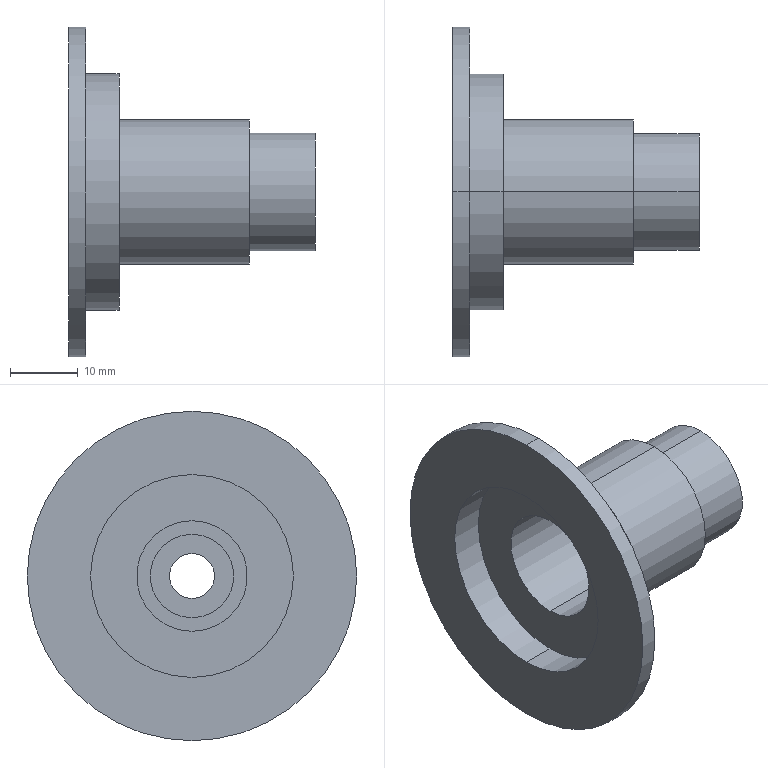Part | SolidWorks | features Revolution 1 | 1 solid | 24 faces | box 36.357 x 48.558 x 48.558 mm | volume 9786 mm3 | cylinder 16 | plane 8 | commonest cylinder face diameters 6.627 x2 12.319 x2 16.319 x2 17.319 x2 21.319 x2 29.909 x2
STEP:
#1=CARTESIAN_POINT('',(74.143,0.,-17.455));
#2=VERTEX_POINT('',#1);
#3=CARTESIAN_POINT('',(74.143,0.,17.455));
#4=VERTEX_POINT('',#3);
#5=CARTESIAN_POINT('',(74.143,0.,0.));
#6=DIRECTION('',(1.,0.,0.));
#7=DIRECTION('',(0.,0.,-1.));
#8=AXIS2_PLACEMENT_3D('',#5,#6,#7);
#9=CIRCLE('',#8,17.455);
#10=EDGE_CURVE('',#2,#4,#9,.T.);
#11=ORIENTED_EDGE('',*,*,#10,.T.);
#12=CARTESIAN_POINT('',(79.061,0.,17.455));
#13=VERTEX_POINT('',#12);
#14=CARTESIAN_POINT('',(0.,0.,17.455));
#15=DIRECTION('',(1.,0.,0.));
#16=VECTOR('',#15,1000.);
#17=LINE('',#14,#16);
#18=EDGE_CURVE('',#4,#13,#17,.T.);
#19=ORIENTED_EDGE('',*,*,#18,.T.);
#20=CARTESIAN_POINT('',(79.061,0.,-17.455));
#21=VERTEX_POINT('',#20);
#22=CARTESIAN_POINT('',(79.061,0.,0.));
#23=DIRECTION('',(1.,0.,0.));
#24=DIRECTION('',(0.,0.,-1.));
#25=AXIS2_PLACEMENT_3D('',#22,#23,#24);
#26=CIRCLE('',#25,17.455);
#27=EDGE_CURVE('',#21,#13,#26,.T.);
#28=ORIENTED_EDGE('',*,*,#27,.F.);
#29=CARTESIAN_POINT('',(0.,0.,-17.455));
#30=DIRECTION('',(1.,0.,0.));
#31=VECTOR('',#30,1000.);
#32=LINE('',#29,#31);
#33=EDGE_CURVE('',#2,#21,#32,.T.);
#34=ORIENTED_EDGE('',*,*,#33,.F.);
#35=EDGE_LOOP('',(#11,#19,#28,#34));
#36=FACE_OUTER_BOUND('',#35,.T.);
#37=CARTESIAN_POINT('',(0.,0.,0.));
#38=DIRECTION('',(1.,0.,0.));
#39=DIRECTION('',(0.,0.,-1.));
#40=AXIS2_PLACEMENT_3D('',#37,#38,#39);
#41=CYLINDRICAL_SURFACE('',#40,17.455);
#42=ADVANCED_FACE('',(#36),#41,.T.);
#43=CARTESIAN_POINT('',(79.061,0.,-10.66));
#44=VERTEX_POINT('',#43);
#45=CARTESIAN_POINT('',(79.061,0.,10.66));
#46=VERTEX_POINT('',#45);
#47=CARTESIAN_POINT('',(79.061,0.,0.));
#48=DIRECTION('',(1.,0.,0.));
#49=DIRECTION('',(0.,0.,-1.));
#50=AXIS2_PLACEMENT_3D('',#47,#48,#49);
#51=CIRCLE('',#50,10.66);
#52=EDGE_CURVE('',#44,#46,#51,.T.);
#53=ORIENTED_EDGE('',*,*,#52,.T.);
#54=CARTESIAN_POINT('',(98.286,0.,10.66));
#55=VERTEX_POINT('',#54);
#56=CARTESIAN_POINT('',(0.,0.,10.66));
#57=DIRECTION('',(1.,0.,0.));
#58=VECTOR('',#57,1000.);
#59=LINE('',#56,#58);
#60=EDGE_CURVE('',#46,#55,#59,.T.);
#61=ORIENTED_EDGE('',*,*,#60,.T.);
#62=CARTESIAN_POINT('',(98.286,0.,-10.66));
#63=VERTEX_POINT('',#62);
#64=CARTESIAN_POINT('',(98.286,0.,0.));
#65=DIRECTION('',(1.,0.,0.));
#66=DIRECTION('',(0.,0.,-1.));
#67=AXIS2_PLACEMENT_3D('',#64,#65,#66);
#68=CIRCLE('',#67,10.66);
#69=EDGE_CURVE('',#63,#55,#68,.T.);
#70=ORIENTED_EDGE('',*,*,#69,.F.);
#71=CARTESIAN_POINT('',(0.,0.,-10.66));
#72=DIRECTION('',(1.,0.,0.));
#73=VECTOR('',#72,1000.);
#74=LINE('',#71,#73);
#75=EDGE_CURVE('',#44,#63,#74,.T.);
#76=ORIENTED_EDGE('',*,*,#75,.F.);
#77=EDGE_LOOP('',(#53,#61,#70,#76));
#78=FACE_OUTER_BOUND('',#77,.T.);
#79=CARTESIAN_POINT('',(0.,0.,0.));
#80=DIRECTION('',(1.,0.,0.));
#81=DIRECTION('',(0.,0.,-1.));
#82=AXIS2_PLACEMENT_3D('',#79,#80,#81);
#83=CYLINDRICAL_SURFACE('',#82,10.66);
#84=ADVANCED_FACE('',(#78),#83,.T.);
#85=CARTESIAN_POINT('',(98.286,0.,-8.66));
#86=VERTEX_POINT('',#85);
#87=CARTESIAN_POINT('',(98.286,0.,8.66));
#88=VERTEX_POINT('',#87);
#89=CARTESIAN_POINT('',(98.286,0.,0.));
#90=DIRECTION('',(1.,0.,0.));
#91=DIRECTION('',(0.,0.,-1.));
#92=AXIS2_PLACEMENT_3D('',#89,#90,#91);
#93=CIRCLE('',#92,8.66);
#94=EDGE_CURVE('',#86,#88,#93,.T.);
#95=ORIENTED_EDGE('',*,*,#94,.T.);
#96=CARTESIAN_POINT('',(108.,0.,8.66));
#97=VERTEX_POINT('',#96);
#98=CARTESIAN_POINT('',(0.,0.,8.66));
#99=DIRECTION('',(1.,0.,0.));
#100=VECTOR('',#99,1000.);
#101=LINE('',#98,#100);
#102=EDGE_CURVE('',#88,#97,#101,.T.);
#103=ORIENTED_EDGE('',*,*,#102,.T.);
#104=CARTESIAN_POINT('',(108.,0.,-8.66));
#105=VERTEX_POINT('',#104);
#106=CARTESIAN_POINT('',(108.,0.,0.));
#107=DIRECTION('',(1.,0.,0.));
#108=DIRECTION('',(0.,0.,-1.));
#109=AXIS2_PLACEMENT_3D('',#106,#107,#108);
#110=CIRCLE('',#109,8.66);
#111=EDGE_CURVE('',#105,#97,#110,.T.);
#112=ORIENTED_EDGE('',*,*,#111,.F.);
#113=CARTESIAN_POINT('',(0.,0.,-8.66));
#114=DIRECTION('',(1.,0.,0.));
#115=VECTOR('',#114,1000.);
#116=LINE('',#113,#115);
#117=EDGE_CURVE('',#86,#105,#116,.T.);
#118=ORIENTED_EDGE('',*,*,#117,.F.);
#119=EDGE_LOOP('',(#95,#103,#112,#118));
#120=FACE_OUTER_BOUND('',#119,.T.);
#121=CARTESIAN_POINT('',(0.,0.,0.));
#122=DIRECTION('',(1.,0.,0.));
#123=DIRECTION('',(0.,0.,-1.));
#124=AXIS2_PLACEMENT_3D('',#121,#122,#123);
#125=CYLINDRICAL_SURFACE('',#124,8.66);
#126=ADVANCED_FACE('',(#120),#125,.T.);
#127=CARTESIAN_POINT('',(105.278,0.,3.314));
#128=VERTEX_POINT('',#127);
#129=CARTESIAN_POINT('',(105.278,0.,-3.314));
#130=VERTEX_POINT('',#129);
#131=CARTESIAN_POINT('',(105.278,0.,0.));
#132=DIRECTION('',(1.,0.,0.));
#133=DIRECTION('',(0.,0.,-1.));
#134=AXIS2_PLACEMENT_3D('',#131,#132,#133);
#135=CIRCLE('',#134,3.314);
#136=EDGE_CURVE('',#128,#130,#135,.T.);
#137=ORIENTED_EDGE('',*,*,#136,.F.);
#138=CARTESIAN_POINT('',(108.,0.,3.314));
#139=VERTEX_POINT('',#138);
#140=CARTESIAN_POINT('',(0.,0.,3.314));
#141=DIRECTION('',(1.,0.,0.));
#142=VECTOR('',#141,1000.);
#143=LINE('',#140,#142);
#144=EDGE_CURVE('',#128,#139,#143,.T.);
#145=ORIENTED_EDGE('',*,*,#144,.T.);
#146=CARTESIAN_POINT('',(108.,0.,-3.314));
#147=VERTEX_POINT('',#146);
#148=CARTESIAN_POINT('',(108.,0.,0.));
#149=DIRECTION('',(1.,0.,0.));
#150=DIRECTION('',(0.,0.,-1.));
#151=AXIS2_PLACEMENT_3D('',#148,#149,#150);
#152=CIRCLE('',#151,3.314);
#153=EDGE_CURVE('',#139,#147,#152,.T.);
#154=ORIENTED_EDGE('',*,*,#153,.T.);
#155=CARTESIAN_POINT('',(0.,0.,-3.314));
#156=DIRECTION('',(1.,0.,0.));
#157=VECTOR('',#156,1000.);
#158=LINE('',#155,#157);
#159=EDGE_CURVE('',#130,#147,#158,.T.);
#160=ORIENTED_EDGE('',*,*,#159,.F.);
#161=EDGE_LOOP('',(#137,#145,#154,#160));
#162=FACE_OUTER_BOUND('',#161,.T.);
#163=CARTESIAN_POINT('',(0.,0.,0.));
#164=DIRECTION('',(1.,0.,0.));
#165=DIRECTION('',(0.,0.,-1.));
#166=AXIS2_PLACEMENT_3D('',#163,#164,#165);
#167=CYLINDRICAL_SURFACE('',#166,3.314);
#168=ADVANCED_FACE('',(#162),#167,.F.);
#169=CARTESIAN_POINT('',(95.786,0.,6.16));
#170=VERTEX_POINT('',#169);
#171=CARTESIAN_POINT('',(95.786,0.,-6.16));
#172=VERTEX_POINT('',#171);
#173=CARTESIAN_POINT('',(95.786,0.,0.));
#174=DIRECTION('',(1.,0.,0.));
#175=DIRECTION('',(0.,0.,-1.));
#176=AXIS2_PLACEMENT_3D('',#173,#174,#175);
#177=CIRCLE('',#176,6.16);
#178=EDGE_CURVE('',#170,#172,#177,.T.);
#179=ORIENTED_EDGE('',*,*,#178,.F.);
#180=CARTESIAN_POINT('',(105.278,0.,6.16));
#181=VERTEX_POINT('',#180);
#182=CARTESIAN_POINT('',(0.,0.,6.16));
#183=DIRECTION('',(1.,0.,0.));
#184=VECTOR('',#183,1000.);
#185=LINE('',#182,#184);
#186=EDGE_CURVE('',#170,#181,#185,.T.);
#187=ORIENTED_EDGE('',*,*,#186,.T.);
#188=CARTESIAN_POINT('',(105.278,0.,-6.16));
#189=VERTEX_POINT('',#188);
#190=CARTESIAN_POINT('',(105.278,0.,0.));
#191=DIRECTION('',(1.,0.,0.));
#192=DIRECTION('',(0.,0.,-1.));
#193=AXIS2_PLACEMENT_3D('',#190,#191,#192);
#194=CIRCLE('',#193,6.16);
#195=EDGE_CURVE('',#181,#189,#194,.T.);
#196=ORIENTED_EDGE('',*,*,#195,.T.);
#197=CARTESIAN_POINT('',(0.,0.,-6.16));
#198=DIRECTION('',(1.,0.,0.));
#199=VECTOR('',#198,1000.);
#200=LINE('',#197,#199);
#201=EDGE_CURVE('',#172,#189,#200,.T.);
#202=ORIENTED_EDGE('',*,*,#201,.F.);
#203=EDGE_LOOP('',(#179,#187,#196,#202));
#204=FACE_OUTER_BOUND('',#203,.T.);
#205=CARTESIAN_POINT('',(0.,0.,0.));
#206=DIRECTION('',(1.,0.,0.));
#207=DIRECTION('',(0.,0.,-1.));
#208=AXIS2_PLACEMENT_3D('',#205,#206,#207);
#209=CYLINDRICAL_SURFACE('',#208,6.16);
#210=ADVANCED_FACE('',(#204),#209,.F.);
#211=CARTESIAN_POINT('',(76.561,0.,8.16));
#212=VERTEX_POINT('',#211);
#213=CARTESIAN_POINT('',(76.561,0.,-8.16));
#214=VERTEX_POINT('',#213);
#215=CARTESIAN_POINT('',(76.561,0.,0.));
#216=DIRECTION('',(1.,0.,0.));
#217=DIRECTION('',(0.,0.,-1.));
#218=AXIS2_PLACEMENT_3D('',#215,#216,#217);
#219=CIRCLE('',#218,8.16);
#220=EDGE_CURVE('',#212,#214,#219,.T.);
#221=ORIENTED_EDGE('',*,*,#220,.F.);
#222=CARTESIAN_POINT('',(95.786,0.,8.16));
#223=VERTEX_POINT('',#222);
#224=CARTESIAN_POINT('',(0.,0.,8.16));
#225=DIRECTION('',(1.,0.,0.));
#226=VECTOR('',#225,1000.);
#227=LINE('',#224,#226);
#228=EDGE_CURVE('',#212,#223,#227,.T.);
#229=ORIENTED_EDGE('',*,*,#228,.T.);
#230=CARTESIAN_POINT('',(95.786,0.,-8.16));
#231=VERTEX_POINT('',#230);
#232=CARTESIAN_POINT('',(95.786,0.,0.));
#233=DIRECTION('',(1.,0.,0.));
#234=DIRECTION('',(0.,0.,-1.));
#235=AXIS2_PLACEMENT_3D('',#232,#233,#234);
#236=CIRCLE('',#235,8.16);
#237=EDGE_CURVE('',#223,#231,#236,.T.);
#238=ORIENTED_EDGE('',*,*,#237,.T.);
#239=CARTESIAN_POINT('',(0.,0.,-8.16));
#240=DIRECTION('',(1.,0.,0.));
#241=VECTOR('',#240,1000.);
#242=LINE('',#239,#241);
#243=EDGE_CURVE('',#214,#231,#242,.T.);
#244=ORIENTED_EDGE('',*,*,#243,.F.);
#245=EDGE_LOOP('',(#221,#229,#238,#244));
#246=FACE_OUTER_BOUND('',#245,.T.);
#247=CARTESIAN_POINT('',(0.,0.,0.));
#248=DIRECTION('',(1.,0.,0.));
#249=DIRECTION('',(0.,0.,-1.));
#250=AXIS2_PLACEMENT_3D('',#247,#248,#249);
#251=CYLINDRICAL_SURFACE('',#250,8.16);
#252=ADVANCED_FACE('',(#246),#251,.F.);
#253=CARTESIAN_POINT('',(71.643,0.,14.955));
#254=VERTEX_POINT('',#253);
#255=CARTESIAN_POINT('',(71.643,0.,-14.955));
#256=VERTEX_POINT('',#255);
#257=CARTESIAN_POINT('',(71.643,0.,0.));
#258=DIRECTION('',(1.,0.,0.));
#259=DIRECTION('',(0.,0.,-1.));
#260=AXIS2_PLACEMENT_3D('',#257,#258,#259);
#261=CIRCLE('',#260,14.955);
#262=EDGE_CURVE('',#254,#256,#261,.T.);
#263=ORIENTED_EDGE('',*,*,#262,.F.);
#264=CARTESIAN_POINT('',(76.561,0.,14.955));
#265=VERTEX_POINT('',#264);
#266=CARTESIAN_POINT('',(0.,0.,14.955));
#267=DIRECTION('',(1.,0.,0.));
#268=VECTOR('',#267,1000.);
#269=LINE('',#266,#268);
#270=EDGE_CURVE('',#254,#265,#269,.T.);
#271=ORIENTED_EDGE('',*,*,#270,.T.);
#272=CARTESIAN_POINT('',(76.561,0.,-14.955));
#273=VERTEX_POINT('',#272);
#274=CARTESIAN_POINT('',(76.561,0.,0.));
#275=DIRECTION('',(1.,0.,0.));
#276=DIRECTION('',(0.,0.,-1.));
#277=AXIS2_PLACEMENT_3D('',#274,#275,#276);
#278=CIRCLE('',#277,14.955);
#279=EDGE_CURVE('',#265,#273,#278,.T.);
#280=ORIENTED_EDGE('',*,*,#279,.T.);
#281=CARTESIAN_POINT('',(0.,0.,-14.955));
#282=DIRECTION('',(1.,0.,0.));
#283=VECTOR('',#282,1000.);
#284=LINE('',#281,#283);
#285=EDGE_CURVE('',#256,#273,#284,.T.);
#286=ORIENTED_EDGE('',*,*,#285,.F.);
#287=EDGE_LOOP('',(#263,#271,#280,#286));
#288=FACE_OUTER_BOUND('',#287,.T.);
#289=CARTESIAN_POINT('',(0.,0.,0.));
#290=DIRECTION('',(1.,0.,0.));
#291=DIRECTION('',(0.,0.,-1.));
#292=AXIS2_PLACEMENT_3D('',#289,#290,#291);
#293=CYLINDRICAL_SURFACE('',#292,14.955);
#294=ADVANCED_FACE('',(#288),#293,.F.);
#295=CARTESIAN_POINT('',(71.643,0.,-24.279));
#296=VERTEX_POINT('',#295);
#297=CARTESIAN_POINT('',(71.643,0.,24.279));
#298=VERTEX_POINT('',#297);
#299=CARTESIAN_POINT('',(71.643,0.,0.));
#300=DIRECTION('',(1.,0.,0.));
#301=DIRECTION('',(0.,0.,-1.));
#302=AXIS2_PLACEMENT_3D('',#299,#300,#301);
#303=CIRCLE('',#302,24.279);
#304=EDGE_CURVE('',#296,#298,#303,.T.);
#305=ORIENTED_EDGE('',*,*,#304,.T.);
#306=CARTESIAN_POINT('',(74.143,0.,24.279));
#307=VERTEX_POINT('',#306);
#308=CARTESIAN_POINT('',(0.,0.,24.279));
#309=DIRECTION('',(1.,0.,0.));
#310=VECTOR('',#309,1000.);
#311=LINE('',#308,#310);
#312=EDGE_CURVE('',#298,#307,#311,.T.);
#313=ORIENTED_EDGE('',*,*,#312,.T.);
#314=CARTESIAN_POINT('',(74.143,0.,-24.279));
#315=VERTEX_POINT('',#314);
#316=CARTESIAN_POINT('',(74.143,0.,0.));
#317=DIRECTION('',(1.,0.,0.));
#318=DIRECTION('',(0.,0.,-1.));
#319=AXIS2_PLACEMENT_3D('',#316,#317,#318);
#320=CIRCLE('',#319,24.279);
#321=EDGE_CURVE('',#315,#307,#320,.T.);
#322=ORIENTED_EDGE('',*,*,#321,.F.);
#323=CARTESIAN_POINT('',(0.,0.,-24.279));
#324=DIRECTION('',(1.,0.,0.));
#325=VECTOR('',#324,1000.);
#326=LINE('',#323,#325);
#327=EDGE_CURVE('',#296,#315,#326,.T.);
#328=ORIENTED_EDGE('',*,*,#327,.F.);
#329=EDGE_LOOP('',(#305,#313,#322,#328));
#330=FACE_OUTER_BOUND('',#329,.T.);
#331=CARTESIAN_POINT('',(0.,0.,0.));
#332=DIRECTION('',(1.,0.,0.));
#333=DIRECTION('',(0.,0.,-1.));
#334=AXIS2_PLACEMENT_3D('',#331,#332,#333);
#335=CYLINDRICAL_SURFACE('',#334,24.279);
#336=ADVANCED_FACE('',(#330),#335,.T.);
#337=ORIENTED_EDGE('',*,*,#10,.F.);
#338=CARTESIAN_POINT('',(74.143,0.,0.));
#339=DIRECTION('',(1.,0.,0.));
#340=DIRECTION('',(0.,0.,-1.));
#341=AXIS2_PLACEMENT_3D('',#338,#339,#340);
#342=CIRCLE('',#341,17.455);
#343=EDGE_CURVE('',#4,#2,#342,.T.);
#344=ORIENTED_EDGE('',*,*,#343,.F.);
#345=EDGE_LOOP('',(#337,#344));
#346=FACE_BOUND('',#345,.T.);
#347=ORIENTED_EDGE('',*,*,#321,.T.);
#348=CARTESIAN_POINT('',(74.143,0.,0.));
#349=DIRECTION('',(1.,0.,0.));
#350=DIRECTION('',(0.,0.,-1.));
#351=AXIS2_PLACEMENT_3D('',#348,#349,#350);
#352=CIRCLE('',#351,24.279);
#353=EDGE_CURVE('',#307,#315,#352,.T.);
#354=ORIENTED_EDGE('',*,*,#353,.T.);
#355=EDGE_LOOP('',(#347,#354));
#356=FACE_OUTER_BOUND('',#355,.T.);
#357=CARTESIAN_POINT('',(74.143,0.,0.));
#358=DIRECTION('',(-1.,0.,0.));
#359=DIRECTION('',(0.,0.,1.));
#360=AXIS2_PLACEMENT_3D('',#357,#358,#359);
#361=PLANE('',#360);
#362=ADVANCED_FACE('',(#346,#356),#361,.F.);
#363=ORIENTED_EDGE('',*,*,#312,.F.);
#364=CARTESIAN_POINT('',(71.643,0.,0.));
#365=DIRECTION('',(1.,0.,0.));
#366=DIRECTION('',(0.,0.,-1.));
#367=AXIS2_PLACEMENT_3D('',#364,#365,#366);
#368=CIRCLE('',#367,24.279);
#369=EDGE_CURVE('',#298,#296,#368,.T.);
#370=ORIENTED_EDGE('',*,*,#369,.T.);
#371=ORIENTED_EDGE('',*,*,#327,.T.);
#372=ORIENTED_EDGE('',*,*,#353,.F.);
#373=EDGE_LOOP('',(#363,#370,#371,#372));
#374=FACE_OUTER_BOUND('',#373,.T.);
#375=CARTESIAN_POINT('',(0.,0.,0.));
#376=DIRECTION('',(1.,0.,0.));
#377=DIRECTION('',(0.,0.,-1.));
#378=AXIS2_PLACEMENT_3D('',#375,#376,#377);
#379=CYLINDRICAL_SURFACE('',#378,24.279);
#380=ADVANCED_FACE('',(#374),#379,.T.);
#381=CARTESIAN_POINT('',(71.643,0.,0.));
#382=DIRECTION('',(1.,0.,0.));
#383=DIRECTION('',(0.,0.,-1.));
#384=AXIS2_PLACEMENT_3D('',#381,#382,#383);
#385=CIRCLE('',#384,14.955);
#386=EDGE_CURVE('',#256,#254,#385,.T.);
#387=ORIENTED_EDGE('',*,*,#386,.T.);
#388=ORIENTED_EDGE('',*,*,#262,.T.);
#389=EDGE_LOOP('',(#387,#388));
#390=FACE_BOUND('',#389,.T.);
#391=ORIENTED_EDGE('',*,*,#304,.F.);
#392=ORIENTED_EDGE('',*,*,#369,.F.);
#393=EDGE_LOOP('',(#391,#392));
#394=FACE_OUTER_BOUND('',#393,.T.);
#395=CARTESIAN_POINT('',(71.643,0.,0.));
#396=DIRECTION('',(-1.,0.,0.));
#397=DIRECTION('',(0.,0.,1.));
#398=AXIS2_PLACEMENT_3D('',#395,#396,#397);
#399=PLANE('',#398);
#400=ADVANCED_FACE('',(#390,#394),#399,.T.);
#401=ORIENTED_EDGE('',*,*,#270,.F.);
#402=ORIENTED_EDGE('',*,*,#386,.F.);
#403=ORIENTED_EDGE('',*,*,#285,.T.);
#404=CARTESIAN_POINT('',(76.561,0.,0.));
#405=DIRECTION('',(1.,0.,0.));
#406=DIRECTION('',(0.,0.,-1.));
#407=AXIS2_PLACEMENT_3D('',#404,#405,#406);
#408=CIRCLE('',#407,14.955);
#409=EDGE_CURVE('',#273,#265,#408,.T.);
#410=ORIENTED_EDGE('',*,*,#409,.T.);
#411=EDGE_LOOP('',(#401,#402,#403,#410));
#412=FACE_OUTER_BOUND('',#411,.T.);
#413=CARTESIAN_POINT('',(0.,0.,0.));
#414=DIRECTION('',(1.,0.,0.));
#415=DIRECTION('',(0.,0.,-1.));
#416=AXIS2_PLACEMENT_3D('',#413,#414,#415);
#417=CYLINDRICAL_SURFACE('',#416,14.955);
#418=ADVANCED_FACE('',(#412),#417,.F.);
#419=CARTESIAN_POINT('',(76.561,0.,0.));
#420=DIRECTION('',(1.,0.,0.));
#421=DIRECTION('',(0.,0.,-1.));
#422=AXIS2_PLACEMENT_3D('',#419,#420,#421);
#423=CIRCLE('',#422,8.16);
#424=EDGE_CURVE('',#214,#212,#423,.T.);
#425=ORIENTED_EDGE('',*,*,#424,.T.);
#426=ORIENTED_EDGE('',*,*,#220,.T.);
#427=EDGE_LOOP('',(#425,#426));
#428=FACE_BOUND('',#427,.T.);
#429=ORIENTED_EDGE('',*,*,#409,.F.);
#430=ORIENTED_EDGE('',*,*,#279,.F.);
#431=EDGE_LOOP('',(#429,#430));
#432=FACE_OUTER_BOUND('',#431,.T.);
#433=CARTESIAN_POINT('',(76.561,0.,0.));
#434=DIRECTION('',(-1.,0.,0.));
#435=DIRECTION('',(0.,0.,1.));
#436=AXIS2_PLACEMENT_3D('',#433,#434,#435);
#437=PLANE('',#436);
#438=ADVANCED_FACE('',(#428,#432),#437,.T.);
#439=ORIENTED_EDGE('',*,*,#228,.F.);
#440=ORIENTED_EDGE('',*,*,#424,.F.);
#441=ORIENTED_EDGE('',*,*,#243,.T.);
#442=CARTESIAN_POINT('',(95.786,0.,0.));
#443=DIRECTION('',(1.,0.,0.));
#444=DIRECTION('',(0.,0.,-1.));
#445=AXIS2_PLACEMENT_3D('',#442,#443,#444);
#446=CIRCLE('',#445,8.16);
#447=EDGE_CURVE('',#231,#223,#446,.T.);
#448=ORIENTED_EDGE('',*,*,#447,.T.);
#449=EDGE_LOOP('',(#439,#440,#441,#448));
#450=FACE_OUTER_BOUND('',#449,.T.);
#451=CARTESIAN_POINT('',(0.,0.,0.));
#452=DIRECTION('',(1.,0.,0.));
#453=DIRECTION('',(0.,0.,-1.));
#454=AXIS2_PLACEMENT_3D('',#451,#452,#453);
#455=CYLINDRICAL_SURFACE('',#454,8.16);
#456=ADVANCED_FACE('',(#450),#455,.F.);
#457=CARTESIAN_POINT('',(95.786,0.,0.));
#458=DIRECTION('',(1.,0.,0.));
#459=DIRECTION('',(0.,0.,-1.));
#460=AXIS2_PLACEMENT_3D('',#457,#458,#459);
#461=CIRCLE('',#460,6.16);
#462=EDGE_CURVE('',#172,#170,#461,.T.);
#463=ORIENTED_EDGE('',*,*,#462,.T.);
#464=ORIENTED_EDGE('',*,*,#178,.T.);
#465=EDGE_LOOP('',(#463,#464));
#466=FACE_BOUND('',#465,.T.);
#467=ORIENTED_EDGE('',*,*,#447,.F.);
#468=ORIENTED_EDGE('',*,*,#237,.F.);
#469=EDGE_LOOP('',(#467,#468));
#470=FACE_OUTER_BOUND('',#469,.T.);
#471=CARTESIAN_POINT('',(95.786,0.,0.));
#472=DIRECTION('',(-1.,0.,0.));
#473=DIRECTION('',(0.,0.,1.));
#474=AXIS2_PLACEMENT_3D('',#471,#472,#473);
#475=PLANE('',#474);
#476=ADVANCED_FACE('',(#466,#470),#475,.T.);
#477=ORIENTED_EDGE('',*,*,#186,.F.);
#478=ORIENTED_EDGE('',*,*,#462,.F.);
#479=ORIENTED_EDGE('',*,*,#201,.T.);
#480=CARTESIAN_POINT('',(105.278,0.,0.));
#481=DIRECTION('',(1.,0.,0.));
#482=DIRECTION('',(0.,0.,-1.));
#483=AXIS2_PLACEMENT_3D('',#480,#481,#482);
#484=CIRCLE('',#483,6.16);
#485=EDGE_CURVE('',#189,#181,#484,.T.);
#486=ORIENTED_EDGE('',*,*,#485,.T.);
#487=EDGE_LOOP('',(#477,#478,#479,#486));
#488=FACE_OUTER_BOUND('',#487,.T.);
#489=CARTESIAN_POINT('',(0.,0.,0.));
#490=DIRECTION('',(1.,0.,0.));
#491=DIRECTION('',(0.,0.,-1.));
#492=AXIS2_PLACEMENT_3D('',#489,#490,#491);
#493=CYLINDRICAL_SURFACE('',#492,6.16);
#494=ADVANCED_FACE('',(#488),#493,.F.);
#495=ORIENTED_EDGE('',*,*,#485,.F.);
#496=ORIENTED_EDGE('',*,*,#195,.F.);
#497=EDGE_LOOP('',(#495,#496));
#498=FACE_OUTER_BOUND('',#497,.T.);
#499=CARTESIAN_POINT('',(105.278,0.,0.));
#500=DIRECTION('',(1.,0.,0.));
#501=DIRECTION('',(0.,0.,-1.));
#502=AXIS2_PLACEMENT_3D('',#499,#500,#501);
#503=CIRCLE('',#502,3.314);
#504=EDGE_CURVE('',#130,#128,#503,.T.);
#505=ORIENTED_EDGE('',*,*,#504,.T.);
#506=ORIENTED_EDGE('',*,*,#136,.T.);
#507=EDGE_LOOP('',(#505,#506));
#508=FACE_BOUND('',#507,.T.);
#509=CARTESIAN_POINT('',(105.278,0.,0.));
#510=DIRECTION('',(1.,0.,0.));
#511=DIRECTION('',(0.,0.,-1.));
#512=AXIS2_PLACEMENT_3D('',#509,#510,#511);
#513=PLANE('',#512);
#514=ADVANCED_FACE('',(#498,#508),#513,.F.);
#515=ORIENTED_EDGE('',*,*,#144,.F.);
#516=ORIENTED_EDGE('',*,*,#504,.F.);
#517=ORIENTED_EDGE('',*,*,#159,.T.);
#518=CARTESIAN_POINT('',(108.,0.,0.));
#519=DIRECTION('',(1.,0.,0.));
#520=DIRECTION('',(0.,0.,-1.));
#521=AXIS2_PLACEMENT_3D('',#518,#519,#520);
#522=CIRCLE('',#521,3.314);
#523=EDGE_CURVE('',#147,#139,#522,.T.);
#524=ORIENTED_EDGE('',*,*,#523,.T.);
#525=EDGE_LOOP('',(#515,#516,#517,#524));
#526=FACE_OUTER_BOUND('',#525,.T.);
#527=CARTESIAN_POINT('',(0.,0.,0.));
#528=DIRECTION('',(1.,0.,0.));
#529=DIRECTION('',(0.,0.,-1.));
#530=AXIS2_PLACEMENT_3D('',#527,#528,#529);
#531=CYLINDRICAL_SURFACE('',#530,3.314);
#532=ADVANCED_FACE('',(#526),#531,.F.);
#533=ORIENTED_EDGE('',*,*,#523,.F.);
#534=ORIENTED_EDGE('',*,*,#153,.F.);
#535=EDGE_LOOP('',(#533,#534));
#536=FACE_BOUND('',#535,.T.);
#537=ORIENTED_EDGE('',*,*,#111,.T.);
#538=CARTESIAN_POINT('',(108.,0.,0.));
#539=DIRECTION('',(1.,0.,0.));
#540=DIRECTION('',(0.,0.,-1.));
#541=AXIS2_PLACEMENT_3D('',#538,#539,#540);
#542=CIRCLE('',#541,8.66);
#543=EDGE_CURVE('',#97,#105,#542,.T.);
#544=ORIENTED_EDGE('',*,*,#543,.T.);
#545=EDGE_LOOP('',(#537,#544));
#546=FACE_OUTER_BOUND('',#545,.T.);
#547=CARTESIAN_POINT('',(108.,0.,0.));
#548=DIRECTION('',(-1.,0.,0.));
#549=DIRECTION('',(0.,0.,1.));
#550=AXIS2_PLACEMENT_3D('',#547,#548,#549);
#551=PLANE('',#550);
#552=ADVANCED_FACE('',(#536,#546),#551,.F.);
#553=ORIENTED_EDGE('',*,*,#102,.F.);
#554=CARTESIAN_POINT('',(98.286,0.,0.));
#555=DIRECTION('',(1.,0.,0.));
#556=DIRECTION('',(0.,0.,-1.));
#557=AXIS2_PLACEMENT_3D('',#554,#555,#556);
#558=CIRCLE('',#557,8.66);
#559=EDGE_CURVE('',#88,#86,#558,.T.);
#560=ORIENTED_EDGE('',*,*,#559,.T.);
#561=ORIENTED_EDGE('',*,*,#117,.T.);
#562=ORIENTED_EDGE('',*,*,#543,.F.);
#563=EDGE_LOOP('',(#553,#560,#561,#562));
#564=FACE_OUTER_BOUND('',#563,.T.);
#565=CARTESIAN_POINT('',(0.,0.,0.));
#566=DIRECTION('',(1.,0.,0.));
#567=DIRECTION('',(0.,0.,-1.));
#568=AXIS2_PLACEMENT_3D('',#565,#566,#567);
#569=CYLINDRICAL_SURFACE('',#568,8.66);
#570=ADVANCED_FACE('',(#564),#569,.T.);
#571=ORIENTED_EDGE('',*,*,#94,.F.);
#572=ORIENTED_EDGE('',*,*,#559,.F.);
#573=EDGE_LOOP('',(#571,#572));
#574=FACE_BOUND('',#573,.T.);
#575=ORIENTED_EDGE('',*,*,#69,.T.);
#576=CARTESIAN_POINT('',(98.286,0.,0.));
#577=DIRECTION('',(1.,0.,0.));
#578=DIRECTION('',(0.,0.,-1.));
#579=AXIS2_PLACEMENT_3D('',#576,#577,#578);
#580=CIRCLE('',#579,10.66);
#581=EDGE_CURVE('',#55,#63,#580,.T.);
#582=ORIENTED_EDGE('',*,*,#581,.T.);
#583=EDGE_LOOP('',(#575,#582));
#584=FACE_OUTER_BOUND('',#583,.T.);
#585=CARTESIAN_POINT('',(98.286,0.,0.));
#586=DIRECTION('',(-1.,0.,0.));
#587=DIRECTION('',(0.,0.,1.));
#588=AXIS2_PLACEMENT_3D('',#585,#586,#587);
#589=PLANE('',#588);
#590=ADVANCED_FACE('',(#574,#584),#589,.F.);
#591=ORIENTED_EDGE('',*,*,#60,.F.);
#592=CARTESIAN_POINT('',(79.061,0.,0.));
#593=DIRECTION('',(1.,0.,0.));
#594=DIRECTION('',(0.,0.,-1.));
#595=AXIS2_PLACEMENT_3D('',#592,#593,#594);
#596=CIRCLE('',#595,10.66);
#597=EDGE_CURVE('',#46,#44,#596,.T.);
#598=ORIENTED_EDGE('',*,*,#597,.T.);
#599=ORIENTED_EDGE('',*,*,#75,.T.);
#600=ORIENTED_EDGE('',*,*,#581,.F.);
#601=EDGE_LOOP('',(#591,#598,#599,#600));
#602=FACE_OUTER_BOUND('',#601,.T.);
#603=CARTESIAN_POINT('',(0.,0.,0.));
#604=DIRECTION('',(1.,0.,0.));
#605=DIRECTION('',(0.,0.,-1.));
#606=AXIS2_PLACEMENT_3D('',#603,#604,#605);
#607=CYLINDRICAL_SURFACE('',#606,10.66);
#608=ADVANCED_FACE('',(#602),#607,.T.);
#609=ORIENTED_EDGE('',*,*,#52,.F.);
#610=ORIENTED_EDGE('',*,*,#597,.F.);
#611=EDGE_LOOP('',(#609,#610));
#612=FACE_BOUND('',#611,.T.);
#613=ORIENTED_EDGE('',*,*,#27,.T.);
#614=CARTESIAN_POINT('',(79.061,0.,0.));
#615=DIRECTION('',(1.,0.,0.));
#616=DIRECTION('',(0.,0.,-1.));
#617=AXIS2_PLACEMENT_3D('',#614,#615,#616);
#618=CIRCLE('',#617,17.455);
#619=EDGE_CURVE('',#13,#21,#618,.T.);
#620=ORIENTED_EDGE('',*,*,#619,.T.);
#621=EDGE_LOOP('',(#613,#620));
#622=FACE_OUTER_BOUND('',#621,.T.);
#623=CARTESIAN_POINT('',(79.061,0.,0.));
#624=DIRECTION('',(-1.,0.,0.));
#625=DIRECTION('',(0.,0.,1.));
#626=AXIS2_PLACEMENT_3D('',#623,#624,#625);
#627=PLANE('',#626);
#628=ADVANCED_FACE('',(#612,#622),#627,.F.);
#629=ORIENTED_EDGE('',*,*,#18,.F.);
#630=ORIENTED_EDGE('',*,*,#343,.T.);
#631=ORIENTED_EDGE('',*,*,#33,.T.);
#632=ORIENTED_EDGE('',*,*,#619,.F.);
#633=EDGE_LOOP('',(#629,#630,#631,#632));
#634=FACE_OUTER_BOUND('',#633,.T.);
#635=CARTESIAN_POINT('',(0.,0.,0.));
#636=DIRECTION('',(1.,0.,0.));
#637=DIRECTION('',(0.,0.,-1.));
#638=AXIS2_PLACEMENT_3D('',#635,#636,#637);
#639=CYLINDRICAL_SURFACE('',#638,17.455);
#640=ADVANCED_FACE('',(#634),#639,.T.);
#641=CLOSED_SHELL('',(#42,#84,#126,#168,#210,#252,#294,#336,#362,#380,#400,#418,#438,#456,#476,#494,#514,#532,#552,#570,#590,#608,#628,#640));
#642=MANIFOLD_SOLID_BREP('',#641);
#643=CARTESIAN_POINT('',(0.,0.,0.));
#644=DIRECTION('',(0.,0.,1.));
#645=DIRECTION('',(1.,0.,0.));
#646=AXIS2_PLACEMENT_3D('',#643,#644,#645);
#647=(LENGTH_UNIT()NAMED_UNIT(*)SI_UNIT(.MILLI.,.METRE.));
#648=UNCERTAINTY_MEASURE_WITH_UNIT(LENGTH_MEASURE(0.00001),#647,'','');
#649=(NAMED_UNIT(*)PLANE_ANGLE_UNIT()SI_UNIT($,.RADIAN.));
#650=(NAMED_UNIT(*)SI_UNIT($,.STERADIAN.)SOLID_ANGLE_UNIT());
#651=(GEOMETRIC_REPRESENTATION_CONTEXT(3)GLOBAL_UNCERTAINTY_ASSIGNED_CONTEXT((#648))GLOBAL_UNIT_ASSIGNED_CONTEXT((#647,#649,#650))REPRESENTATION_CONTEXT('',''));
#652=ADVANCED_BREP_SHAPE_REPRESENTATION('',(#642,#646),#651);